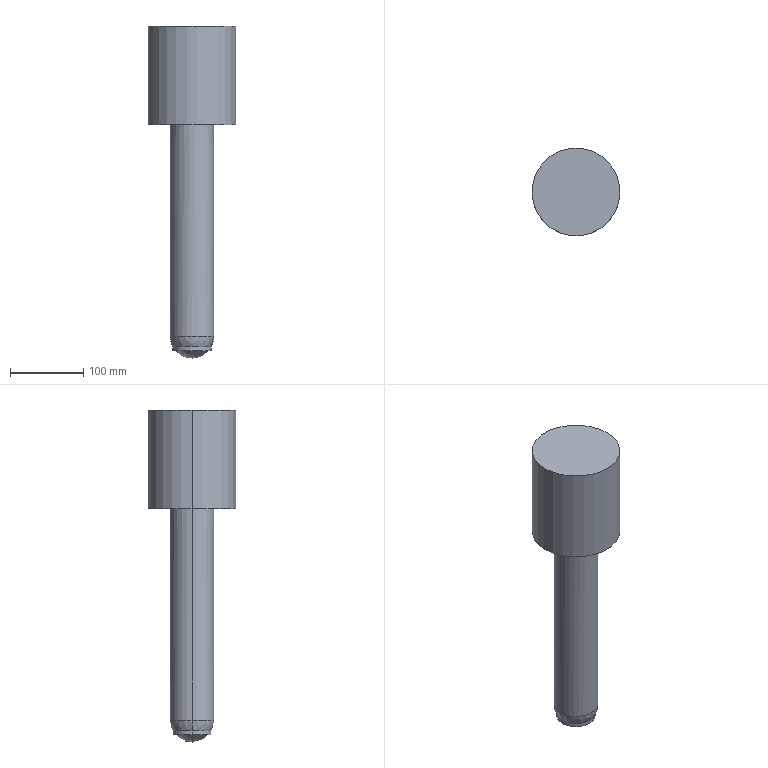Part | SolidWorks | features ICE 2, Extrusion 1, Fillet 1 | 1 solid | 13 faces | box 120 x 120 x 453 mm | volume 2398988 mm3 | cylinder 6 | sphere 4 | plane 3 | commonest cylinder face diameters 52 x2 60 x2 120 x2
STEP:
#1=CARTESIAN_POINT('',(577.524,0.,-443.));
#2=VERTEX_POINT('',#1);
#3=CARTESIAN_POINT('',(622.245,0.,-443.));
#4=VERTEX_POINT('',#3);
#5=CARTESIAN_POINT('',(599.884,0.,-443.));
#6=DIRECTION('',(0.,0.,-1.));
#7=DIRECTION('',(1.,0.,0.));
#8=AXIS2_PLACEMENT_3D('',#5,#6,#7);
#9=CIRCLE('',#8,22.361);
#10=EDGE_CURVE('',#2,#4,#9,.T.);
#11=ORIENTED_EDGE('',*,*,#10,.T.);
#12=CARTESIAN_POINT('',(599.884,0.,-453.));
#13=VERTEX_POINT('',#12);
#14=CARTESIAN_POINT('',(599.884,0.,-423.));
#15=DIRECTION('',(0.,1.,0.));
#16=DIRECTION('',(-1.,0.,0.));
#17=AXIS2_PLACEMENT_3D('',#14,#15,#16);
#18=CIRCLE('',#17,30.);
#19=EDGE_CURVE('',#4,#13,#18,.T.);
#20=ORIENTED_EDGE('',*,*,#19,.T.);
#21=CARTESIAN_POINT('',(599.884,0.,-423.));
#22=DIRECTION('',(0.,-1.,0.));
#23=DIRECTION('',(0.,0.,-1.));
#24=AXIS2_PLACEMENT_3D('',#21,#22,#23);
#25=CIRCLE('',#24,30.);
#26=EDGE_CURVE('',#2,#13,#25,.T.);
#27=ORIENTED_EDGE('',*,*,#26,.F.);
#28=EDGE_LOOP('',(#11,#20,#27));
#29=FACE_OUTER_BOUND('',#28,.T.);
#30=CARTESIAN_POINT('',(599.884,0.,-423.));
#31=DIRECTION('',(0.,1.,0.));
#32=DIRECTION('',(-1.,0.,0.));
#33=AXIS2_PLACEMENT_3D('',#30,#31,#32);
#34=SPHERICAL_SURFACE('',#33,30.);
#35=ADVANCED_FACE('',(#29),#34,.T.);
#36=CARTESIAN_POINT('',(625.884,0.,-443.));
#37=VERTEX_POINT('',#36);
#38=CARTESIAN_POINT('',(573.884,0.,-443.));
#39=VERTEX_POINT('',#38);
#40=CARTESIAN_POINT('',(599.884,0.,-443.));
#41=DIRECTION('',(0.,0.,1.));
#42=DIRECTION('',(1.,0.,0.));
#43=AXIS2_PLACEMENT_3D('',#40,#41,#42);
#44=CIRCLE('',#43,26.);
#45=EDGE_CURVE('',#37,#39,#44,.T.);
#46=ORIENTED_EDGE('',*,*,#45,.T.);
#47=CARTESIAN_POINT('',(573.884,0.,-437.967));
#48=VERTEX_POINT('',#47);
#49=CARTESIAN_POINT('',(573.884,0.,-443.));
#50=DIRECTION('',(0.,0.,1.));
#51=VECTOR('',#50,1000.);
#52=LINE('',#49,#51);
#53=EDGE_CURVE('',#39,#48,#52,.T.);
#54=ORIENTED_EDGE('',*,*,#53,.T.);
#55=CARTESIAN_POINT('',(625.884,0.,-437.967));
#56=VERTEX_POINT('',#55);
#57=CARTESIAN_POINT('',(599.884,0.,-437.967));
#58=DIRECTION('',(0.,0.,-1.));
#59=DIRECTION('',(1.,0.,0.));
#60=AXIS2_PLACEMENT_3D('',#57,#58,#59);
#61=CIRCLE('',#60,26.);
#62=EDGE_CURVE('',#48,#56,#61,.T.);
#63=ORIENTED_EDGE('',*,*,#62,.T.);
#64=CARTESIAN_POINT('',(625.884,0.,-443.));
#65=DIRECTION('',(0.,0.,1.));
#66=VECTOR('',#65,1000.);
#67=LINE('',#64,#66);
#68=EDGE_CURVE('',#37,#56,#67,.T.);
#69=ORIENTED_EDGE('',*,*,#68,.F.);
#70=EDGE_LOOP('',(#46,#54,#63,#69));
#71=FACE_OUTER_BOUND('',#70,.T.);
#72=CARTESIAN_POINT('',(599.884,0.,-443.));
#73=DIRECTION('',(0.,0.,1.));
#74=DIRECTION('',(1.,0.,0.));
#75=AXIS2_PLACEMENT_3D('',#72,#73,#74);
#76=CYLINDRICAL_SURFACE('',#75,26.);
#77=ADVANCED_FACE('',(#71),#76,.T.);
#78=CARTESIAN_POINT('',(629.884,0.,-423.));
#79=VERTEX_POINT('',#78);
#80=CARTESIAN_POINT('',(569.884,0.,-423.));
#81=VERTEX_POINT('',#80);
#82=CARTESIAN_POINT('',(599.884,0.,-423.));
#83=DIRECTION('',(0.,0.,1.));
#84=DIRECTION('',(1.,0.,0.));
#85=AXIS2_PLACEMENT_3D('',#82,#83,#84);
#86=CIRCLE('',#85,30.);
#87=EDGE_CURVE('',#79,#81,#86,.T.);
#88=ORIENTED_EDGE('',*,*,#87,.F.);
#89=CARTESIAN_POINT('',(599.884,0.,-423.));
#90=DIRECTION('',(0.,1.,0.));
#91=DIRECTION('',(-1.,0.,0.));
#92=AXIS2_PLACEMENT_3D('',#89,#90,#91);
#93=CIRCLE('',#92,30.);
#94=EDGE_CURVE('',#79,#56,#93,.T.);
#95=ORIENTED_EDGE('',*,*,#94,.T.);
#96=ORIENTED_EDGE('',*,*,#62,.F.);
#97=CARTESIAN_POINT('',(599.884,0.,-423.));
#98=DIRECTION('',(0.,-1.,0.));
#99=DIRECTION('',(0.,0.,-1.));
#100=AXIS2_PLACEMENT_3D('',#97,#98,#99);
#101=CIRCLE('',#100,30.);
#102=EDGE_CURVE('',#81,#48,#101,.T.);
#103=ORIENTED_EDGE('',*,*,#102,.F.);
#104=EDGE_LOOP('',(#88,#95,#96,#103));
#105=FACE_OUTER_BOUND('',#104,.T.);
#106=CARTESIAN_POINT('',(599.884,0.,-423.));
#107=DIRECTION('',(0.,1.,0.));
#108=DIRECTION('',(-1.,0.,0.));
#109=AXIS2_PLACEMENT_3D('',#106,#107,#108);
#110=SPHERICAL_SURFACE('',#109,30.);
#111=ADVANCED_FACE('',(#105),#110,.T.);
#112=ORIENTED_EDGE('',*,*,#87,.T.);
#113=CARTESIAN_POINT('',(569.884,0.,-135.));
#114=VERTEX_POINT('',#113);
#115=CARTESIAN_POINT('',(569.884,0.,-453.));
#116=DIRECTION('',(0.,0.,1.));
#117=VECTOR('',#116,1000.);
#118=LINE('',#115,#117);
#119=EDGE_CURVE('',#81,#114,#118,.T.);
#120=ORIENTED_EDGE('',*,*,#119,.T.);
#121=CARTESIAN_POINT('',(629.884,0.,-135.));
#122=VERTEX_POINT('',#121);
#123=CARTESIAN_POINT('',(599.884,0.,-135.));
#124=DIRECTION('',(0.,0.,-1.));
#125=DIRECTION('',(-1.,0.,0.));
#126=AXIS2_PLACEMENT_3D('',#123,#124,#125);
#127=CIRCLE('',#126,30.);
#128=EDGE_CURVE('',#114,#122,#127,.T.);
#129=ORIENTED_EDGE('',*,*,#128,.T.);
#130=CARTESIAN_POINT('',(629.884,0.,-453.));
#131=DIRECTION('',(0.,0.,1.));
#132=VECTOR('',#131,1000.);
#133=LINE('',#130,#132);
#134=EDGE_CURVE('',#79,#122,#133,.T.);
#135=ORIENTED_EDGE('',*,*,#134,.F.);
#136=EDGE_LOOP('',(#112,#120,#129,#135));
#137=FACE_OUTER_BOUND('',#136,.T.);
#138=CARTESIAN_POINT('',(599.884,0.,-453.));
#139=DIRECTION('',(0.,0.,1.));
#140=DIRECTION('',(1.,0.,0.));
#141=AXIS2_PLACEMENT_3D('',#138,#139,#140);
#142=CYLINDRICAL_SURFACE('',#141,30.);
#143=ADVANCED_FACE('',(#137),#142,.T.);
#144=CARTESIAN_POINT('',(659.884,0.,-135.));
#145=VERTEX_POINT('',#144);
#146=CARTESIAN_POINT('',(539.884,0.,-135.));
#147=VERTEX_POINT('',#146);
#148=CARTESIAN_POINT('',(599.884,0.,-135.));
#149=DIRECTION('',(0.,0.,1.));
#150=DIRECTION('',(1.,0.,0.));
#151=AXIS2_PLACEMENT_3D('',#148,#149,#150);
#152=CIRCLE('',#151,60.);
#153=EDGE_CURVE('',#145,#147,#152,.T.);
#154=ORIENTED_EDGE('',*,*,#153,.T.);
#155=CARTESIAN_POINT('',(539.884,0.,0.));
#156=VERTEX_POINT('',#155);
#157=CARTESIAN_POINT('',(539.884,0.,-135.));
#158=DIRECTION('',(0.,0.,1.));
#159=VECTOR('',#158,1000.);
#160=LINE('',#157,#159);
#161=EDGE_CURVE('',#147,#156,#160,.T.);
#162=ORIENTED_EDGE('',*,*,#161,.T.);
#163=CARTESIAN_POINT('',(659.884,0.,0.));
#164=VERTEX_POINT('',#163);
#165=CARTESIAN_POINT('',(599.884,0.,0.));
#166=DIRECTION('',(0.,0.,1.));
#167=DIRECTION('',(1.,0.,0.));
#168=AXIS2_PLACEMENT_3D('',#165,#166,#167);
#169=CIRCLE('',#168,60.);
#170=EDGE_CURVE('',#164,#156,#169,.T.);
#171=ORIENTED_EDGE('',*,*,#170,.F.);
#172=CARTESIAN_POINT('',(659.884,0.,-135.));
#173=DIRECTION('',(0.,0.,1.));
#174=VECTOR('',#173,1000.);
#175=LINE('',#172,#174);
#176=EDGE_CURVE('',#145,#164,#175,.T.);
#177=ORIENTED_EDGE('',*,*,#176,.F.);
#178=EDGE_LOOP('',(#154,#162,#171,#177));
#179=FACE_OUTER_BOUND('',#178,.T.);
#180=CARTESIAN_POINT('',(599.884,0.,-135.));
#181=DIRECTION('',(0.,0.,1.));
#182=DIRECTION('',(1.,0.,0.));
#183=AXIS2_PLACEMENT_3D('',#180,#181,#182);
#184=CYLINDRICAL_SURFACE('',#183,60.);
#185=ADVANCED_FACE('',(#179),#184,.T.);
#186=ORIENTED_EDGE('',*,*,#161,.F.);
#187=CARTESIAN_POINT('',(599.884,0.,-135.));
#188=DIRECTION('',(0.,0.,1.));
#189=DIRECTION('',(1.,0.,0.));
#190=AXIS2_PLACEMENT_3D('',#187,#188,#189);
#191=CIRCLE('',#190,60.);
#192=EDGE_CURVE('',#147,#145,#191,.T.);
#193=ORIENTED_EDGE('',*,*,#192,.T.);
#194=ORIENTED_EDGE('',*,*,#176,.T.);
#195=CARTESIAN_POINT('',(599.884,0.,0.));
#196=DIRECTION('',(0.,0.,1.));
#197=DIRECTION('',(1.,0.,0.));
#198=AXIS2_PLACEMENT_3D('',#195,#196,#197);
#199=CIRCLE('',#198,60.);
#200=EDGE_CURVE('',#156,#164,#199,.T.);
#201=ORIENTED_EDGE('',*,*,#200,.F.);
#202=EDGE_LOOP('',(#186,#193,#194,#201));
#203=FACE_OUTER_BOUND('',#202,.T.);
#204=CARTESIAN_POINT('',(599.884,0.,-135.));
#205=DIRECTION('',(0.,0.,1.));
#206=DIRECTION('',(1.,0.,0.));
#207=AXIS2_PLACEMENT_3D('',#204,#205,#206);
#208=CYLINDRICAL_SURFACE('',#207,60.);
#209=ADVANCED_FACE('',(#203),#208,.T.);
#210=CARTESIAN_POINT('',(599.884,0.,-135.));
#211=DIRECTION('',(0.,0.,-1.));
#212=DIRECTION('',(-1.,0.,0.));
#213=AXIS2_PLACEMENT_3D('',#210,#211,#212);
#214=CIRCLE('',#213,30.);
#215=EDGE_CURVE('',#122,#114,#214,.T.);
#216=ORIENTED_EDGE('',*,*,#215,.F.);
#217=ORIENTED_EDGE('',*,*,#128,.F.);
#218=EDGE_LOOP('',(#216,#217));
#219=FACE_BOUND('',#218,.T.);
#220=ORIENTED_EDGE('',*,*,#153,.F.);
#221=ORIENTED_EDGE('',*,*,#192,.F.);
#222=EDGE_LOOP('',(#220,#221));
#223=FACE_OUTER_BOUND('',#222,.T.);
#224=CARTESIAN_POINT('',(599.884,0.,-135.));
#225=DIRECTION('',(0.,0.,1.));
#226=DIRECTION('',(1.,0.,0.));
#227=AXIS2_PLACEMENT_3D('',#224,#225,#226);
#228=PLANE('',#227);
#229=ADVANCED_FACE('',(#219,#223),#228,.F.);
#230=ORIENTED_EDGE('',*,*,#170,.T.);
#231=ORIENTED_EDGE('',*,*,#200,.T.);
#232=EDGE_LOOP('',(#230,#231));
#233=FACE_OUTER_BOUND('',#232,.T.);
#234=CARTESIAN_POINT('',(599.884,0.,0.));
#235=DIRECTION('',(0.,0.,1.));
#236=DIRECTION('',(1.,0.,0.));
#237=AXIS2_PLACEMENT_3D('',#234,#235,#236);
#238=PLANE('',#237);
#239=ADVANCED_FACE('',(#233),#238,.T.);
#240=ORIENTED_EDGE('',*,*,#119,.F.);
#241=CARTESIAN_POINT('',(599.884,0.,-423.));
#242=DIRECTION('',(0.,0.,1.));
#243=DIRECTION('',(1.,0.,0.));
#244=AXIS2_PLACEMENT_3D('',#241,#242,#243);
#245=CIRCLE('',#244,30.);
#246=EDGE_CURVE('',#81,#79,#245,.T.);
#247=ORIENTED_EDGE('',*,*,#246,.T.);
#248=ORIENTED_EDGE('',*,*,#134,.T.);
#249=ORIENTED_EDGE('',*,*,#215,.T.);
#250=EDGE_LOOP('',(#240,#247,#248,#249));
#251=FACE_OUTER_BOUND('',#250,.T.);
#252=CARTESIAN_POINT('',(599.884,0.,-453.));
#253=DIRECTION('',(0.,0.,1.));
#254=DIRECTION('',(1.,0.,0.));
#255=AXIS2_PLACEMENT_3D('',#252,#253,#254);
#256=CYLINDRICAL_SURFACE('',#255,30.);
#257=ADVANCED_FACE('',(#251),#256,.T.);
#258=ORIENTED_EDGE('',*,*,#94,.F.);
#259=ORIENTED_EDGE('',*,*,#246,.F.);
#260=ORIENTED_EDGE('',*,*,#102,.T.);
#261=CARTESIAN_POINT('',(599.884,0.,-437.967));
#262=DIRECTION('',(0.,0.,-1.));
#263=DIRECTION('',(1.,0.,0.));
#264=AXIS2_PLACEMENT_3D('',#261,#262,#263);
#265=CIRCLE('',#264,26.);
#266=EDGE_CURVE('',#56,#48,#265,.T.);
#267=ORIENTED_EDGE('',*,*,#266,.F.);
#268=EDGE_LOOP('',(#258,#259,#260,#267));
#269=FACE_OUTER_BOUND('',#268,.T.);
#270=CARTESIAN_POINT('',(599.884,0.,-423.));
#271=DIRECTION('',(0.,1.,0.));
#272=DIRECTION('',(-1.,0.,0.));
#273=AXIS2_PLACEMENT_3D('',#270,#271,#272);
#274=SPHERICAL_SURFACE('',#273,30.);
#275=ADVANCED_FACE('',(#269),#274,.T.);
#276=ORIENTED_EDGE('',*,*,#53,.F.);
#277=CARTESIAN_POINT('',(599.884,0.,-443.));
#278=DIRECTION('',(0.,0.,1.));
#279=DIRECTION('',(1.,0.,0.));
#280=AXIS2_PLACEMENT_3D('',#277,#278,#279);
#281=CIRCLE('',#280,26.);
#282=EDGE_CURVE('',#39,#37,#281,.T.);
#283=ORIENTED_EDGE('',*,*,#282,.T.);
#284=ORIENTED_EDGE('',*,*,#68,.T.);
#285=ORIENTED_EDGE('',*,*,#266,.T.);
#286=EDGE_LOOP('',(#276,#283,#284,#285));
#287=FACE_OUTER_BOUND('',#286,.T.);
#288=CARTESIAN_POINT('',(599.884,0.,-443.));
#289=DIRECTION('',(0.,0.,1.));
#290=DIRECTION('',(1.,0.,0.));
#291=AXIS2_PLACEMENT_3D('',#288,#289,#290);
#292=CYLINDRICAL_SURFACE('',#291,26.);
#293=ADVANCED_FACE('',(#287),#292,.T.);
#294=ORIENTED_EDGE('',*,*,#10,.F.);
#295=CARTESIAN_POINT('',(599.884,0.,-443.));
#296=DIRECTION('',(0.,0.,-1.));
#297=DIRECTION('',(1.,0.,0.));
#298=AXIS2_PLACEMENT_3D('',#295,#296,#297);
#299=CIRCLE('',#298,22.361);
#300=EDGE_CURVE('',#4,#2,#299,.T.);
#301=ORIENTED_EDGE('',*,*,#300,.F.);
#302=EDGE_LOOP('',(#294,#301));
#303=FACE_BOUND('',#302,.T.);
#304=ORIENTED_EDGE('',*,*,#45,.F.);
#305=ORIENTED_EDGE('',*,*,#282,.F.);
#306=EDGE_LOOP('',(#304,#305));
#307=FACE_OUTER_BOUND('',#306,.T.);
#308=CARTESIAN_POINT('',(599.884,0.,-443.));
#309=DIRECTION('',(0.,0.,1.));
#310=DIRECTION('',(1.,0.,0.));
#311=AXIS2_PLACEMENT_3D('',#308,#309,#310);
#312=PLANE('',#311);
#313=ADVANCED_FACE('',(#303,#307),#312,.F.);
#314=ORIENTED_EDGE('',*,*,#19,.F.);
#315=ORIENTED_EDGE('',*,*,#300,.T.);
#316=ORIENTED_EDGE('',*,*,#26,.T.);
#317=EDGE_LOOP('',(#314,#315,#316));
#318=FACE_OUTER_BOUND('',#317,.T.);
#319=CARTESIAN_POINT('',(599.884,0.,-423.));
#320=DIRECTION('',(0.,1.,0.));
#321=DIRECTION('',(-1.,0.,0.));
#322=AXIS2_PLACEMENT_3D('',#319,#320,#321);
#323=SPHERICAL_SURFACE('',#322,30.);
#324=ADVANCED_FACE('',(#318),#323,.T.);
#325=CLOSED_SHELL('',(#35,#77,#111,#143,#185,#209,#229,#239,#257,#275,#293,#313,#324));
#326=MANIFOLD_SOLID_BREP('',#325);
#327=CARTESIAN_POINT('',(0.,0.,0.));
#328=DIRECTION('',(0.,0.,1.));
#329=DIRECTION('',(1.,0.,0.));
#330=AXIS2_PLACEMENT_3D('',#327,#328,#329);
#331=(LENGTH_UNIT()NAMED_UNIT(*)SI_UNIT(.MILLI.,.METRE.));
#332=UNCERTAINTY_MEASURE_WITH_UNIT(LENGTH_MEASURE(0.00001),#331,'','');
#333=(NAMED_UNIT(*)PLANE_ANGLE_UNIT()SI_UNIT($,.RADIAN.));
#334=(NAMED_UNIT(*)SI_UNIT($,.STERADIAN.)SOLID_ANGLE_UNIT());
#335=(GEOMETRIC_REPRESENTATION_CONTEXT(3)GLOBAL_UNCERTAINTY_ASSIGNED_CONTEXT((#332))GLOBAL_UNIT_ASSIGNED_CONTEXT((#331,#333,#334))REPRESENTATION_CONTEXT('',''));
#336=ADVANCED_BREP_SHAPE_REPRESENTATION('',(#326,#330),#335);